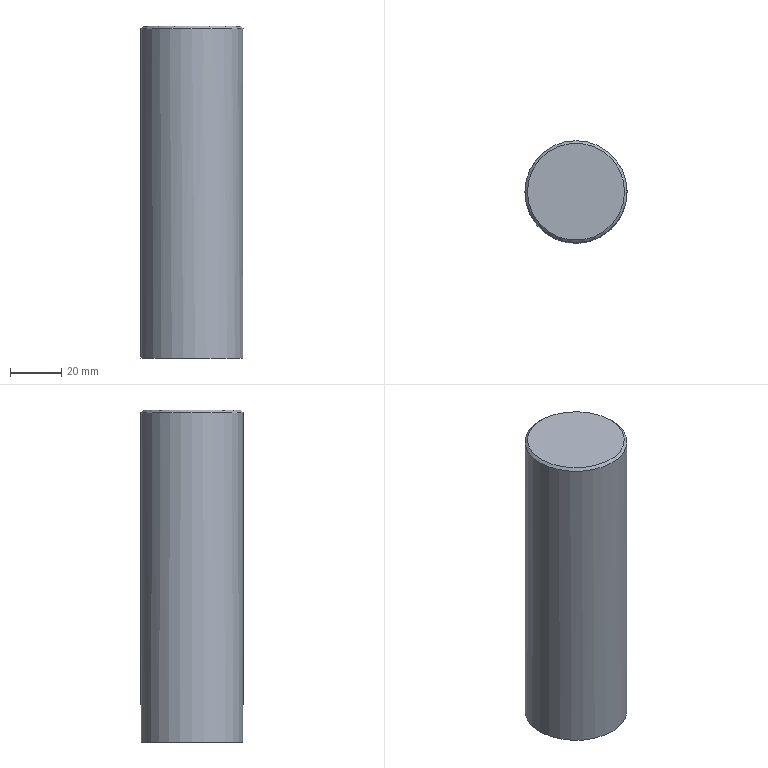Part | STEP file | solid 175 | 1 solid | 6 faces | box 40 x 40 x 130 mm | volume 162047 mm3 | plane 2 | cylinder 2 | cone 2 | commonest cylinder face diameters 10 x1 40 x1